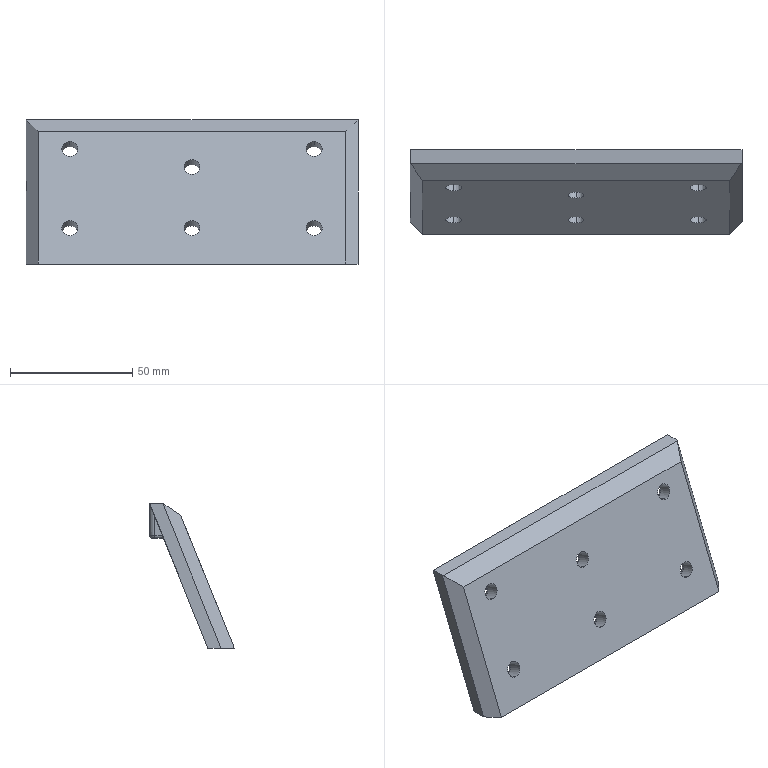Part | Creo | 1 solid | 56 faces | box 136 x 34.623 x 59 mm | volume 81644 mm3 | cylinder 29 | plane 13 | cone 12 | torus 2 | commonest cylinder face diameters 6.6 x12 13 x12 2 x3 4 x2